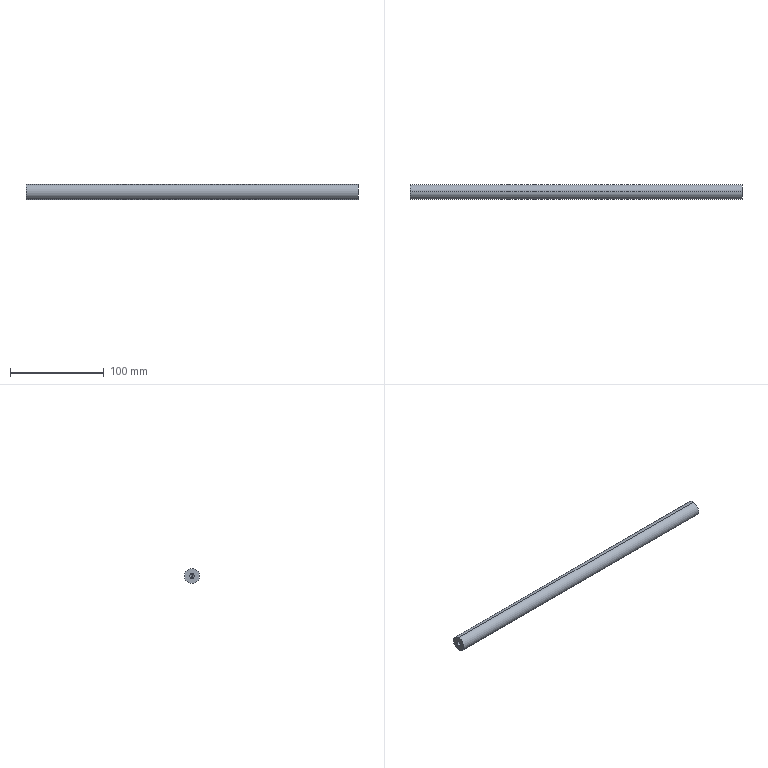Part | SolidWorks | features HoleWzd 2, Revolution 1 | 1 solid | 12 faces | box 354 x 16 x 16 mm | volume 70567 mm3 | cylinder 6 | cone 4 | plane 2 | commonest cylinder face diameters 5 x4 16 x2
STEP:
#1=CARTESIAN_POINT('',(-162.,0.,-2.5));
#2=VERTEX_POINT('',#1);
#3=CARTESIAN_POINT('',(-162.,0.,2.5));
#4=VERTEX_POINT('',#3);
#5=CARTESIAN_POINT('',(-162.,0.,0.));
#6=DIRECTION('',(-1.,0.,0.));
#7=DIRECTION('',(0.,0.,1.));
#8=AXIS2_PLACEMENT_3D('',#5,#6,#7);
#9=CIRCLE('',#8,2.5);
#10=EDGE_CURVE('',#2,#4,#9,.T.);
#11=ORIENTED_EDGE('',*,*,#10,.F.);
#12=CARTESIAN_POINT('',(-177.,0.,-2.5));
#13=VERTEX_POINT('',#12);
#14=CARTESIAN_POINT('',(-177.,0.,-2.5));
#15=DIRECTION('',(-1.,0.,0.));
#16=VECTOR('',#15,1000.);
#17=LINE('',#14,#16);
#18=EDGE_CURVE('',#2,#13,#17,.T.);
#19=ORIENTED_EDGE('',*,*,#18,.T.);
#20=CARTESIAN_POINT('',(-177.,0.,2.5));
#21=VERTEX_POINT('',#20);
#22=CARTESIAN_POINT('',(-177.,0.,0.));
#23=DIRECTION('',(-1.,0.,0.));
#24=DIRECTION('',(0.,0.,1.));
#25=AXIS2_PLACEMENT_3D('',#22,#23,#24);
#26=CIRCLE('',#25,2.5);
#27=EDGE_CURVE('',#13,#21,#26,.T.);
#28=ORIENTED_EDGE('',*,*,#27,.T.);
#29=CARTESIAN_POINT('',(-177.,0.,2.5));
#30=DIRECTION('',(-1.,0.,0.));
#31=VECTOR('',#30,1000.);
#32=LINE('',#29,#31);
#33=EDGE_CURVE('',#4,#21,#32,.T.);
#34=ORIENTED_EDGE('',*,*,#33,.F.);
#35=EDGE_LOOP('',(#11,#19,#28,#34));
#36=FACE_OUTER_BOUND('',#35,.T.);
#37=CARTESIAN_POINT('',(-177.,0.,0.));
#38=DIRECTION('',(-1.,0.,0.));
#39=DIRECTION('',(0.,0.,1.));
#40=AXIS2_PLACEMENT_3D('',#37,#38,#39);
#41=CYLINDRICAL_SURFACE('',#40,2.5);
#42=ADVANCED_FACE('',(#36),#41,.F.);
#43=CARTESIAN_POINT('',(-160.498,0.,0.));
#44=VERTEX_POINT('',#43);
#45=CARTESIAN_POINT('',(-162.,0.,2.5));
#46=DIRECTION('',(-0.515,0.,0.8572));
#47=VECTOR('',#46,1000.);
#48=LINE('',#45,#47);
#49=EDGE_CURVE('',#44,#4,#48,.T.);
#50=ORIENTED_EDGE('',*,*,#49,.F.);
#51=CARTESIAN_POINT('',(-162.,0.,-2.5));
#52=DIRECTION('',(-0.515,0.,-0.8572));
#53=VECTOR('',#52,1000.);
#54=LINE('',#51,#53);
#55=EDGE_CURVE('',#44,#2,#54,.T.);
#56=ORIENTED_EDGE('',*,*,#55,.T.);
#57=ORIENTED_EDGE('',*,*,#10,.T.);
#58=EDGE_LOOP('',(#50,#56,#57));
#59=FACE_OUTER_BOUND('',#58,.T.);
#60=CARTESIAN_POINT('',(-162.,0.,0.));
#61=DIRECTION('',(-1.,0.,0.));
#62=DIRECTION('',(0.,0.,1.));
#63=AXIS2_PLACEMENT_3D('',#60,#61,#62);
#64=CONICAL_SURFACE('',#63,2.5,1.03);
#65=ADVANCED_FACE('',(#59),#64,.F.);
#66=CARTESIAN_POINT('',(162.,0.,2.5));
#67=VERTEX_POINT('',#66);
#68=CARTESIAN_POINT('',(162.,0.,-2.5));
#69=VERTEX_POINT('',#68);
#70=CARTESIAN_POINT('',(162.,0.,0.));
#71=DIRECTION('',(1.,0.,0.));
#72=DIRECTION('',(0.,0.,-1.));
#73=AXIS2_PLACEMENT_3D('',#70,#71,#72);
#74=CIRCLE('',#73,2.5);
#75=EDGE_CURVE('',#67,#69,#74,.T.);
#76=ORIENTED_EDGE('',*,*,#75,.F.);
#77=CARTESIAN_POINT('',(177.,0.,2.5));
#78=VERTEX_POINT('',#77);
#79=CARTESIAN_POINT('',(177.,0.,2.5));
#80=DIRECTION('',(1.,0.,0.));
#81=VECTOR('',#80,1000.);
#82=LINE('',#79,#81);
#83=EDGE_CURVE('',#67,#78,#82,.T.);
#84=ORIENTED_EDGE('',*,*,#83,.T.);
#85=CARTESIAN_POINT('',(177.,0.,-2.5));
#86=VERTEX_POINT('',#85);
#87=CARTESIAN_POINT('',(177.,0.,0.));
#88=DIRECTION('',(1.,0.,0.));
#89=DIRECTION('',(0.,0.,-1.));
#90=AXIS2_PLACEMENT_3D('',#87,#88,#89);
#91=CIRCLE('',#90,2.5);
#92=EDGE_CURVE('',#78,#86,#91,.T.);
#93=ORIENTED_EDGE('',*,*,#92,.T.);
#94=CARTESIAN_POINT('',(177.,0.,-2.5));
#95=DIRECTION('',(1.,0.,0.));
#96=VECTOR('',#95,1000.);
#97=LINE('',#94,#96);
#98=EDGE_CURVE('',#69,#86,#97,.T.);
#99=ORIENTED_EDGE('',*,*,#98,.F.);
#100=EDGE_LOOP('',(#76,#84,#93,#99));
#101=FACE_OUTER_BOUND('',#100,.T.);
#102=CARTESIAN_POINT('',(177.,0.,0.));
#103=DIRECTION('',(1.,0.,0.));
#104=DIRECTION('',(0.,0.,-1.));
#105=AXIS2_PLACEMENT_3D('',#102,#103,#104);
#106=CYLINDRICAL_SURFACE('',#105,2.5);
#107=ADVANCED_FACE('',(#101),#106,.F.);
#108=CARTESIAN_POINT('',(160.498,0.,0.));
#109=VERTEX_POINT('',#108);
#110=CARTESIAN_POINT('',(162.,0.,-2.5));
#111=DIRECTION('',(0.515,0.,-0.8572));
#112=VECTOR('',#111,1000.);
#113=LINE('',#110,#112);
#114=EDGE_CURVE('',#109,#69,#113,.T.);
#115=ORIENTED_EDGE('',*,*,#114,.F.);
#116=CARTESIAN_POINT('',(162.,0.,2.5));
#117=DIRECTION('',(0.515,0.,0.8572));
#118=VECTOR('',#117,1000.);
#119=LINE('',#116,#118);
#120=EDGE_CURVE('',#109,#67,#119,.T.);
#121=ORIENTED_EDGE('',*,*,#120,.T.);
#122=ORIENTED_EDGE('',*,*,#75,.T.);
#123=EDGE_LOOP('',(#115,#121,#122));
#124=FACE_OUTER_BOUND('',#123,.T.);
#125=CARTESIAN_POINT('',(162.,0.,0.));
#126=DIRECTION('',(1.,0.,0.));
#127=DIRECTION('',(0.,0.,-1.));
#128=AXIS2_PLACEMENT_3D('',#125,#126,#127);
#129=CONICAL_SURFACE('',#128,2.5,1.03);
#130=ADVANCED_FACE('',(#124),#129,.F.);
#131=CARTESIAN_POINT('',(177.,0.,8.));
#132=VERTEX_POINT('',#131);
#133=CARTESIAN_POINT('',(177.,0.,-8.));
#134=VERTEX_POINT('',#133);
#135=CARTESIAN_POINT('',(177.,0.,0.));
#136=DIRECTION('',(-1.,0.,0.));
#137=DIRECTION('',(0.,0.,1.));
#138=AXIS2_PLACEMENT_3D('',#135,#136,#137);
#139=CIRCLE('',#138,8.);
#140=EDGE_CURVE('',#132,#134,#139,.T.);
#141=ORIENTED_EDGE('',*,*,#140,.T.);
#142=CARTESIAN_POINT('',(-177.,0.,-8.));
#143=VERTEX_POINT('',#142);
#144=CARTESIAN_POINT('',(-177.,0.,-8.));
#145=DIRECTION('',(-1.,0.,0.));
#146=VECTOR('',#145,1000.);
#147=LINE('',#144,#146);
#148=EDGE_CURVE('',#134,#143,#147,.T.);
#149=ORIENTED_EDGE('',*,*,#148,.T.);
#150=CARTESIAN_POINT('',(-177.,0.,8.));
#151=VERTEX_POINT('',#150);
#152=CARTESIAN_POINT('',(-177.,0.,0.));
#153=DIRECTION('',(-1.,0.,0.));
#154=DIRECTION('',(0.,0.,1.));
#155=AXIS2_PLACEMENT_3D('',#152,#153,#154);
#156=CIRCLE('',#155,8.);
#157=EDGE_CURVE('',#151,#143,#156,.T.);
#158=ORIENTED_EDGE('',*,*,#157,.F.);
#159=CARTESIAN_POINT('',(-177.,0.,8.));
#160=DIRECTION('',(-1.,0.,0.));
#161=VECTOR('',#160,1000.);
#162=LINE('',#159,#161);
#163=EDGE_CURVE('',#132,#151,#162,.T.);
#164=ORIENTED_EDGE('',*,*,#163,.F.);
#165=EDGE_LOOP('',(#141,#149,#158,#164));
#166=FACE_OUTER_BOUND('',#165,.T.);
#167=CARTESIAN_POINT('',(-177.,0.,0.));
#168=DIRECTION('',(-1.,0.,0.));
#169=DIRECTION('',(0.,0.,1.));
#170=AXIS2_PLACEMENT_3D('',#167,#168,#169);
#171=CYLINDRICAL_SURFACE('',#170,8.);
#172=ADVANCED_FACE('',(#166),#171,.T.);
#173=CARTESIAN_POINT('',(-177.,0.,0.));
#174=DIRECTION('',(-1.,0.,0.));
#175=DIRECTION('',(0.,0.,1.));
#176=AXIS2_PLACEMENT_3D('',#173,#174,#175);
#177=CIRCLE('',#176,2.5);
#178=EDGE_CURVE('',#21,#13,#177,.T.);
#179=ORIENTED_EDGE('',*,*,#178,.F.);
#180=ORIENTED_EDGE('',*,*,#27,.F.);
#181=EDGE_LOOP('',(#179,#180));
#182=FACE_BOUND('',#181,.T.);
#183=ORIENTED_EDGE('',*,*,#157,.T.);
#184=CARTESIAN_POINT('',(-177.,0.,0.));
#185=DIRECTION('',(-1.,0.,0.));
#186=DIRECTION('',(0.,0.,1.));
#187=AXIS2_PLACEMENT_3D('',#184,#185,#186);
#188=CIRCLE('',#187,8.);
#189=EDGE_CURVE('',#143,#151,#188,.T.);
#190=ORIENTED_EDGE('',*,*,#189,.T.);
#191=EDGE_LOOP('',(#183,#190));
#192=FACE_OUTER_BOUND('',#191,.T.);
#193=CARTESIAN_POINT('',(-177.,8.,0.));
#194=DIRECTION('',(1.,0.,0.));
#195=DIRECTION('',(0.,0.,-1.));
#196=AXIS2_PLACEMENT_3D('',#193,#194,#195);
#197=PLANE('',#196);
#198=ADVANCED_FACE('',(#182,#192),#197,.F.);
#199=ORIENTED_EDGE('',*,*,#148,.F.);
#200=CARTESIAN_POINT('',(177.,0.,0.));
#201=DIRECTION('',(-1.,0.,0.));
#202=DIRECTION('',(0.,0.,1.));
#203=AXIS2_PLACEMENT_3D('',#200,#201,#202);
#204=CIRCLE('',#203,8.);
#205=EDGE_CURVE('',#134,#132,#204,.T.);
#206=ORIENTED_EDGE('',*,*,#205,.T.);
#207=ORIENTED_EDGE('',*,*,#163,.T.);
#208=ORIENTED_EDGE('',*,*,#189,.F.);
#209=EDGE_LOOP('',(#199,#206,#207,#208));
#210=FACE_OUTER_BOUND('',#209,.T.);
#211=CARTESIAN_POINT('',(-177.,0.,0.));
#212=DIRECTION('',(-1.,0.,0.));
#213=DIRECTION('',(0.,0.,1.));
#214=AXIS2_PLACEMENT_3D('',#211,#212,#213);
#215=CYLINDRICAL_SURFACE('',#214,8.);
#216=ADVANCED_FACE('',(#210),#215,.T.);
#217=CARTESIAN_POINT('',(177.,0.,0.));
#218=DIRECTION('',(1.,0.,0.));
#219=DIRECTION('',(0.,0.,-1.));
#220=AXIS2_PLACEMENT_3D('',#217,#218,#219);
#221=CIRCLE('',#220,2.5);
#222=EDGE_CURVE('',#86,#78,#221,.T.);
#223=ORIENTED_EDGE('',*,*,#222,.F.);
#224=ORIENTED_EDGE('',*,*,#92,.F.);
#225=EDGE_LOOP('',(#223,#224));
#226=FACE_BOUND('',#225,.T.);
#227=ORIENTED_EDGE('',*,*,#140,.F.);
#228=ORIENTED_EDGE('',*,*,#205,.F.);
#229=EDGE_LOOP('',(#227,#228));
#230=FACE_OUTER_BOUND('',#229,.T.);
#231=CARTESIAN_POINT('',(177.,8.,0.));
#232=DIRECTION('',(-1.,0.,0.));
#233=DIRECTION('',(0.,0.,1.));
#234=AXIS2_PLACEMENT_3D('',#231,#232,#233);
#235=PLANE('',#234);
#236=ADVANCED_FACE('',(#226,#230),#235,.F.);
#237=ORIENTED_EDGE('',*,*,#120,.F.);
#238=ORIENTED_EDGE('',*,*,#114,.T.);
#239=CARTESIAN_POINT('',(162.,0.,0.));
#240=DIRECTION('',(1.,0.,0.));
#241=DIRECTION('',(0.,0.,-1.));
#242=AXIS2_PLACEMENT_3D('',#239,#240,#241);
#243=CIRCLE('',#242,2.5);
#244=EDGE_CURVE('',#69,#67,#243,.T.);
#245=ORIENTED_EDGE('',*,*,#244,.T.);
#246=EDGE_LOOP('',(#237,#238,#245));
#247=FACE_OUTER_BOUND('',#246,.T.);
#248=CARTESIAN_POINT('',(162.,0.,0.));
#249=DIRECTION('',(1.,0.,0.));
#250=DIRECTION('',(0.,0.,-1.));
#251=AXIS2_PLACEMENT_3D('',#248,#249,#250);
#252=CONICAL_SURFACE('',#251,2.5,1.03);
#253=ADVANCED_FACE('',(#247),#252,.F.);
#254=ORIENTED_EDGE('',*,*,#83,.F.);
#255=ORIENTED_EDGE('',*,*,#244,.F.);
#256=ORIENTED_EDGE('',*,*,#98,.T.);
#257=ORIENTED_EDGE('',*,*,#222,.T.);
#258=EDGE_LOOP('',(#254,#255,#256,#257));
#259=FACE_OUTER_BOUND('',#258,.T.);
#260=CARTESIAN_POINT('',(177.,0.,0.));
#261=DIRECTION('',(1.,0.,0.));
#262=DIRECTION('',(0.,0.,-1.));
#263=AXIS2_PLACEMENT_3D('',#260,#261,#262);
#264=CYLINDRICAL_SURFACE('',#263,2.5);
#265=ADVANCED_FACE('',(#259),#264,.F.);
#266=ORIENTED_EDGE('',*,*,#55,.F.);
#267=ORIENTED_EDGE('',*,*,#49,.T.);
#268=CARTESIAN_POINT('',(-162.,0.,0.));
#269=DIRECTION('',(-1.,0.,0.));
#270=DIRECTION('',(0.,0.,1.));
#271=AXIS2_PLACEMENT_3D('',#268,#269,#270);
#272=CIRCLE('',#271,2.5);
#273=EDGE_CURVE('',#4,#2,#272,.T.);
#274=ORIENTED_EDGE('',*,*,#273,.T.);
#275=EDGE_LOOP('',(#266,#267,#274));
#276=FACE_OUTER_BOUND('',#275,.T.);
#277=CARTESIAN_POINT('',(-162.,0.,0.));
#278=DIRECTION('',(-1.,0.,0.));
#279=DIRECTION('',(0.,0.,1.));
#280=AXIS2_PLACEMENT_3D('',#277,#278,#279);
#281=CONICAL_SURFACE('',#280,2.5,1.03);
#282=ADVANCED_FACE('',(#276),#281,.F.);
#283=ORIENTED_EDGE('',*,*,#18,.F.);
#284=ORIENTED_EDGE('',*,*,#273,.F.);
#285=ORIENTED_EDGE('',*,*,#33,.T.);
#286=ORIENTED_EDGE('',*,*,#178,.T.);
#287=EDGE_LOOP('',(#283,#284,#285,#286));
#288=FACE_OUTER_BOUND('',#287,.T.);
#289=CARTESIAN_POINT('',(-177.,0.,0.));
#290=DIRECTION('',(-1.,0.,0.));
#291=DIRECTION('',(0.,0.,1.));
#292=AXIS2_PLACEMENT_3D('',#289,#290,#291);
#293=CYLINDRICAL_SURFACE('',#292,2.5);
#294=ADVANCED_FACE('',(#288),#293,.F.);
#295=CLOSED_SHELL('',(#42,#65,#107,#130,#172,#198,#216,#236,#253,#265,#282,#294));
#296=MANIFOLD_SOLID_BREP('',#295);
#297=CARTESIAN_POINT('',(0.,0.,0.));
#298=DIRECTION('',(0.,0.,1.));
#299=DIRECTION('',(1.,0.,0.));
#300=AXIS2_PLACEMENT_3D('',#297,#298,#299);
#301=(LENGTH_UNIT()NAMED_UNIT(*)SI_UNIT(.MILLI.,.METRE.));
#302=UNCERTAINTY_MEASURE_WITH_UNIT(LENGTH_MEASURE(0.00001),#301,'','');
#303=(NAMED_UNIT(*)PLANE_ANGLE_UNIT()SI_UNIT($,.RADIAN.));
#304=(NAMED_UNIT(*)SI_UNIT($,.STERADIAN.)SOLID_ANGLE_UNIT());
#305=(GEOMETRIC_REPRESENTATION_CONTEXT(3)GLOBAL_UNCERTAINTY_ASSIGNED_CONTEXT((#302))GLOBAL_UNIT_ASSIGNED_CONTEXT((#301,#303,#304))REPRESENTATION_CONTEXT('',''));
#306=ADVANCED_BREP_SHAPE_REPRESENTATION('',(#296,#300),#305);